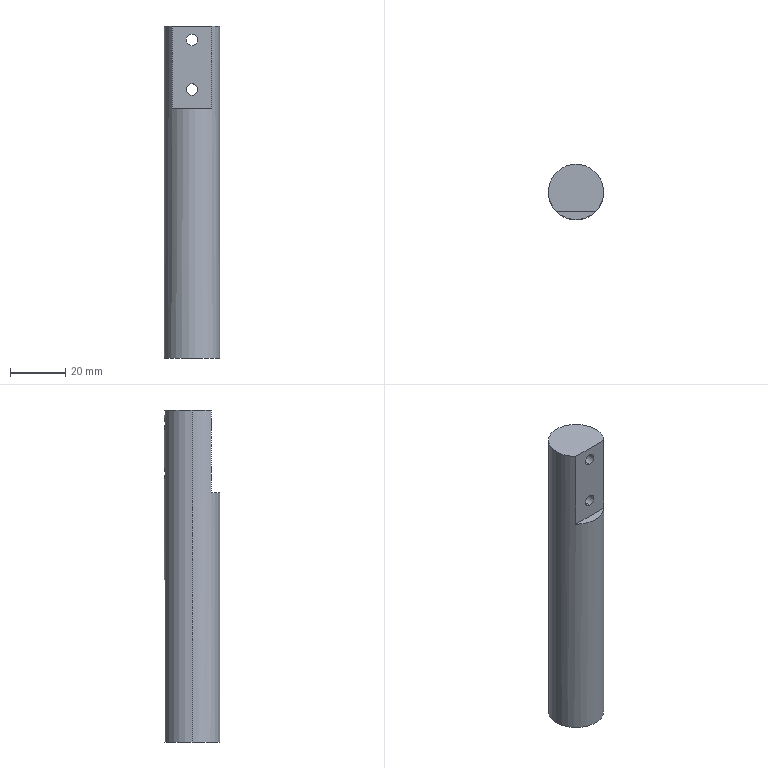Part | SolidWorks | features HoleWzd 2, Extrusion 1, ICE 1 | 1 solid | 14 faces | box 20 x 20 x 120 mm | volume 36039 mm3 | cylinder 8 | plane 4 | cone 2 | commonest cylinder face diameters 4.2 x4 5 x2 20 x2
STEP:
#1=CARTESIAN_POINT('',(0.,10.,57.1));
#2=VERTEX_POINT('',#1);
#3=CARTESIAN_POINT('',(0.,10.,52.9));
#4=VERTEX_POINT('',#3);
#5=CARTESIAN_POINT('',(0.,10.,57.1));
#6=CARTESIAN_POINT('',(-0.2745,10.,57.1));
#7=CARTESIAN_POINT('',(-0.5515,9.988,57.045));
#8=CARTESIAN_POINT('',(-0.9307,9.957,56.887));
#9=CARTESIAN_POINT('',(-1.053,9.945,56.822));
#10=CARTESIAN_POINT('',(-1.282,9.918,56.669));
#11=CARTESIAN_POINT('',(-1.387,9.904,56.582));
#12=CARTESIAN_POINT('',(-1.581,9.875,56.389));
#13=CARTESIAN_POINT('',(-1.669,9.86,56.281));
#14=CARTESIAN_POINT('',(-1.821,9.833,56.054));
#15=CARTESIAN_POINT('',(-1.886,9.821,55.934));
#16=CARTESIAN_POINT('',(-2.045,9.789,55.551));
#17=CARTESIAN_POINT('',(-2.1,9.777,55.278));
#18=CARTESIAN_POINT('',(-2.1,9.777,54.862));
#19=CARTESIAN_POINT('',(-2.087,9.78,54.726));
#20=CARTESIAN_POINT('',(-2.033,9.791,54.457));
#21=CARTESIAN_POINT('',(-1.992,9.8,54.323));
#22=CARTESIAN_POINT('',(-1.887,9.82,54.069));
#23=CARTESIAN_POINT('',(-1.823,9.833,53.948));
#24=CARTESIAN_POINT('',(-1.67,9.86,53.72));
#25=CARTESIAN_POINT('',(-1.582,9.875,53.613));
#26=CARTESIAN_POINT('',(-1.293,9.918,53.323));
#27=CARTESIAN_POINT('',(-1.06,9.947,53.166));
#28=CARTESIAN_POINT('',(-0.6807,9.978,53.009));
#29=CARTESIAN_POINT('',(-0.5474,9.986,52.968));
#30=CARTESIAN_POINT('',(-0.2764,9.997,52.914));
#31=CARTESIAN_POINT('',(-0.1391,10.,52.9));
#32=CARTESIAN_POINT('',(0.,10.,52.9));
#33=B_SPLINE_CURVE_WITH_KNOTS('',3,(#5,#6,#7,#8,#9,#10,#11,#12,#13,#14,#15,#16,#17,#18,#19,#20,#21,#22,#23,#24,#25,#26,#27,#28,#29,#30,#31,#32),.UNSPECIFIED.,.F.,.F.,(4,2,2,2,2,2,2,2,2,2,2,2,2,4),(0.006584,0.007407,0.007818,0.008229,0.008641,0.009052,0.009875,0.01029,0.0107,0.01111,0.01152,0.01234,0.01275,0.01317),.UNSPECIFIED.);
#34=EDGE_CURVE('',#2,#4,#33,.T.);
#35=ORIENTED_EDGE('',*,*,#34,.F.);
#36=CARTESIAN_POINT('',(0.,-7.,57.1));
#37=VERTEX_POINT('',#36);
#38=CARTESIAN_POINT('',(0.,-7.,57.1));
#39=DIRECTION('',(0.,-1.,0.));
#40=VECTOR('',#39,1000.);
#41=LINE('',#38,#40);
#42=EDGE_CURVE('',#2,#37,#41,.T.);
#43=ORIENTED_EDGE('',*,*,#42,.T.);
#44=CARTESIAN_POINT('',(0.,-7.,52.9));
#45=VERTEX_POINT('',#44);
#46=CARTESIAN_POINT('',(0.,-7.,55.));
#47=DIRECTION('',(0.,-1.,0.));
#48=DIRECTION('',(0.,0.,-1.));
#49=AXIS2_PLACEMENT_3D('',#46,#47,#48);
#50=CIRCLE('',#49,2.1);
#51=EDGE_CURVE('',#37,#45,#50,.T.);
#52=ORIENTED_EDGE('',*,*,#51,.T.);
#53=CARTESIAN_POINT('',(0.,-7.,52.9));
#54=DIRECTION('',(0.,-1.,0.));
#55=VECTOR('',#54,1000.);
#56=LINE('',#53,#55);
#57=EDGE_CURVE('',#4,#45,#56,.T.);
#58=ORIENTED_EDGE('',*,*,#57,.F.);
#59=EDGE_LOOP('',(#35,#43,#52,#58));
#60=FACE_OUTER_BOUND('',#59,.T.);
#61=CARTESIAN_POINT('',(0.,-7.,55.));
#62=DIRECTION('',(0.,-1.,0.));
#63=DIRECTION('',(0.,0.,-1.));
#64=AXIS2_PLACEMENT_3D('',#61,#62,#63);
#65=CYLINDRICAL_SURFACE('',#64,2.1);
#66=ADVANCED_FACE('',(#60),#65,.F.);
#67=CARTESIAN_POINT('',(0.,10.,39.1));
#68=VERTEX_POINT('',#67);
#69=CARTESIAN_POINT('',(0.,10.,34.9));
#70=VERTEX_POINT('',#69);
#71=CARTESIAN_POINT('',(0.,10.,39.1));
#72=CARTESIAN_POINT('',(-0.2745,10.,39.1));
#73=CARTESIAN_POINT('',(-0.5515,9.988,39.045));
#74=CARTESIAN_POINT('',(-0.9307,9.957,38.887));
#75=CARTESIAN_POINT('',(-1.053,9.945,38.822));
#76=CARTESIAN_POINT('',(-1.282,9.918,38.669));
#77=CARTESIAN_POINT('',(-1.387,9.904,38.582));
#78=CARTESIAN_POINT('',(-1.581,9.875,38.389));
#79=CARTESIAN_POINT('',(-1.669,9.86,38.281));
#80=CARTESIAN_POINT('',(-1.821,9.833,38.054));
#81=CARTESIAN_POINT('',(-1.886,9.821,37.934));
#82=CARTESIAN_POINT('',(-2.045,9.789,37.551));
#83=CARTESIAN_POINT('',(-2.1,9.777,37.278));
#84=CARTESIAN_POINT('',(-2.1,9.777,36.862));
#85=CARTESIAN_POINT('',(-2.087,9.78,36.726));
#86=CARTESIAN_POINT('',(-2.033,9.791,36.457));
#87=CARTESIAN_POINT('',(-1.992,9.8,36.323));
#88=CARTESIAN_POINT('',(-1.887,9.82,36.069));
#89=CARTESIAN_POINT('',(-1.823,9.833,35.948));
#90=CARTESIAN_POINT('',(-1.67,9.86,35.72));
#91=CARTESIAN_POINT('',(-1.582,9.875,35.613));
#92=CARTESIAN_POINT('',(-1.293,9.918,35.323));
#93=CARTESIAN_POINT('',(-1.06,9.947,35.166));
#94=CARTESIAN_POINT('',(-0.6807,9.978,35.009));
#95=CARTESIAN_POINT('',(-0.5474,9.986,34.968));
#96=CARTESIAN_POINT('',(-0.2764,9.997,34.914));
#97=CARTESIAN_POINT('',(-0.1391,10.,34.9));
#98=CARTESIAN_POINT('',(0.,10.,34.9));
#99=B_SPLINE_CURVE_WITH_KNOTS('',3,(#71,#72,#73,#74,#75,#76,#77,#78,#79,#80,#81,#82,#83,#84,#85,#86,#87,#88,#89,#90,#91,#92,#93,#94,#95,#96,#97,#98),.UNSPECIFIED.,.F.,.F.,(4,2,2,2,2,2,2,2,2,2,2,2,2,4),(0.006584,0.007407,0.007818,0.008229,0.008641,0.009052,0.009875,0.01029,0.0107,0.01111,0.01152,0.01234,0.01275,0.01317),.UNSPECIFIED.);
#100=EDGE_CURVE('',#68,#70,#99,.T.);
#101=ORIENTED_EDGE('',*,*,#100,.F.);
#102=CARTESIAN_POINT('',(0.,-7.,39.1));
#103=VERTEX_POINT('',#102);
#104=CARTESIAN_POINT('',(0.,-7.,39.1));
#105=DIRECTION('',(0.,-1.,0.));
#106=VECTOR('',#105,1000.);
#107=LINE('',#104,#106);
#108=EDGE_CURVE('',#68,#103,#107,.T.);
#109=ORIENTED_EDGE('',*,*,#108,.T.);
#110=CARTESIAN_POINT('',(0.,-7.,34.9));
#111=VERTEX_POINT('',#110);
#112=CARTESIAN_POINT('',(0.,-7.,37.));
#113=DIRECTION('',(0.,-1.,0.));
#114=DIRECTION('',(0.,0.,-1.));
#115=AXIS2_PLACEMENT_3D('',#112,#113,#114);
#116=CIRCLE('',#115,2.1);
#117=EDGE_CURVE('',#103,#111,#116,.T.);
#118=ORIENTED_EDGE('',*,*,#117,.T.);
#119=CARTESIAN_POINT('',(0.,-7.,34.9));
#120=DIRECTION('',(0.,-1.,0.));
#121=VECTOR('',#120,1000.);
#122=LINE('',#119,#121);
#123=EDGE_CURVE('',#70,#111,#122,.T.);
#124=ORIENTED_EDGE('',*,*,#123,.F.);
#125=EDGE_LOOP('',(#101,#109,#118,#124));
#126=FACE_OUTER_BOUND('',#125,.T.);
#127=CARTESIAN_POINT('',(0.,-7.,37.));
#128=DIRECTION('',(0.,-1.,0.));
#129=DIRECTION('',(0.,0.,-1.));
#130=AXIS2_PLACEMENT_3D('',#127,#128,#129);
#131=CYLINDRICAL_SURFACE('',#130,2.1);
#132=ADVANCED_FACE('',(#126),#131,.F.);
#133=CARTESIAN_POINT('',(2.5,0.,-45.));
#134=VERTEX_POINT('',#133);
#135=CARTESIAN_POINT('',(-2.5,0.,-45.));
#136=VERTEX_POINT('',#135);
#137=CARTESIAN_POINT('',(0.,0.,-45.));
#138=DIRECTION('',(0.,0.,-1.));
#139=DIRECTION('',(-1.,0.,0.));
#140=AXIS2_PLACEMENT_3D('',#137,#138,#139);
#141=CIRCLE('',#140,2.5);
#142=EDGE_CURVE('',#134,#136,#141,.T.);
#143=ORIENTED_EDGE('',*,*,#142,.F.);
#144=CARTESIAN_POINT('',(2.5,0.,-60.));
#145=VERTEX_POINT('',#144);
#146=CARTESIAN_POINT('',(2.5,0.,-60.));
#147=DIRECTION('',(0.,0.,-1.));
#148=VECTOR('',#147,1000.);
#149=LINE('',#146,#148);
#150=EDGE_CURVE('',#134,#145,#149,.T.);
#151=ORIENTED_EDGE('',*,*,#150,.T.);
#152=CARTESIAN_POINT('',(-2.5,0.,-60.));
#153=VERTEX_POINT('',#152);
#154=CARTESIAN_POINT('',(0.,0.,-60.));
#155=DIRECTION('',(0.,0.,-1.));
#156=DIRECTION('',(-1.,0.,0.));
#157=AXIS2_PLACEMENT_3D('',#154,#155,#156);
#158=CIRCLE('',#157,2.5);
#159=EDGE_CURVE('',#145,#153,#158,.T.);
#160=ORIENTED_EDGE('',*,*,#159,.T.);
#161=CARTESIAN_POINT('',(-2.5,0.,-60.));
#162=DIRECTION('',(0.,0.,-1.));
#163=VECTOR('',#162,1000.);
#164=LINE('',#161,#163);
#165=EDGE_CURVE('',#136,#153,#164,.T.);
#166=ORIENTED_EDGE('',*,*,#165,.F.);
#167=EDGE_LOOP('',(#143,#151,#160,#166));
#168=FACE_OUTER_BOUND('',#167,.T.);
#169=CARTESIAN_POINT('',(0.,0.,-60.));
#170=DIRECTION('',(0.,0.,-1.));
#171=DIRECTION('',(-1.,0.,0.));
#172=AXIS2_PLACEMENT_3D('',#169,#170,#171);
#173=CYLINDRICAL_SURFACE('',#172,2.5);
#174=ADVANCED_FACE('',(#168),#173,.F.);
#175=CARTESIAN_POINT('',(0.,0.,-43.498));
#176=VERTEX_POINT('',#175);
#177=CARTESIAN_POINT('',(-2.5,0.,-45.));
#178=DIRECTION('',(-0.8572,0.,-0.515));
#179=VECTOR('',#178,1000.);
#180=LINE('',#177,#179);
#181=EDGE_CURVE('',#176,#136,#180,.T.);
#182=ORIENTED_EDGE('',*,*,#181,.F.);
#183=CARTESIAN_POINT('',(2.5,0.,-45.));
#184=DIRECTION('',(0.8572,0.,-0.515));
#185=VECTOR('',#184,1000.);
#186=LINE('',#183,#185);
#187=EDGE_CURVE('',#176,#134,#186,.T.);
#188=ORIENTED_EDGE('',*,*,#187,.T.);
#189=ORIENTED_EDGE('',*,*,#142,.T.);
#190=EDGE_LOOP('',(#182,#188,#189));
#191=FACE_OUTER_BOUND('',#190,.T.);
#192=CARTESIAN_POINT('',(0.,0.,-45.));
#193=DIRECTION('',(0.,0.,-1.));
#194=DIRECTION('',(-1.,0.,0.));
#195=AXIS2_PLACEMENT_3D('',#192,#193,#194);
#196=CONICAL_SURFACE('',#195,2.5,1.03);
#197=ADVANCED_FACE('',(#191),#196,.F.);
#198=CARTESIAN_POINT('',(0.,10.,52.9));
#199=CARTESIAN_POINT('',(0.1392,10.,52.9));
#200=CARTESIAN_POINT('',(0.2759,9.997,52.914));
#201=CARTESIAN_POINT('',(0.5449,9.986,52.967));
#202=CARTESIAN_POINT('',(0.6785,9.978,53.008));
#203=CARTESIAN_POINT('',(0.9326,9.957,53.113));
#204=CARTESIAN_POINT('',(1.053,9.945,53.178));
#205=CARTESIAN_POINT('',(1.281,9.918,53.33));
#206=CARTESIAN_POINT('',(1.389,9.904,53.419));
#207=CARTESIAN_POINT('',(1.678,9.86,53.709));
#208=CARTESIAN_POINT('',(1.835,9.831,53.942));
#209=CARTESIAN_POINT('',(1.992,9.8,54.321));
#210=CARTESIAN_POINT('',(2.032,9.791,54.454));
#211=CARTESIAN_POINT('',(2.087,9.78,54.725));
#212=CARTESIAN_POINT('',(2.1,9.777,54.862));
#213=CARTESIAN_POINT('',(2.1,9.777,55.137));
#214=CARTESIAN_POINT('',(2.086,9.78,55.276));
#215=CARTESIAN_POINT('',(2.032,9.791,55.546));
#216=CARTESIAN_POINT('',(1.993,9.8,55.677));
#217=CARTESIAN_POINT('',(1.834,9.831,56.059));
#218=CARTESIAN_POINT('',(1.68,9.86,56.29));
#219=CARTESIAN_POINT('',(1.387,9.904,56.583));
#220=CARTESIAN_POINT('',(1.282,9.918,56.669));
#221=CARTESIAN_POINT('',(1.054,9.945,56.821));
#222=CARTESIAN_POINT('',(0.9314,9.957,56.887));
#223=CARTESIAN_POINT('',(0.6776,9.978,56.992));
#224=CARTESIAN_POINT('',(0.5467,9.986,57.032));
#225=CARTESIAN_POINT('',(0.2767,9.997,57.086));
#226=CARTESIAN_POINT('',(0.1373,10.,57.1));
#227=CARTESIAN_POINT('',(0.,10.,57.1));
#228=B_SPLINE_CURVE_WITH_KNOTS('',3,(#198,#199,#200,#201,#202,#203,#204,#205,#206,#207,#208,#209,#210,#211,#212,#213,#214,#215,#216,#217,#218,#219,#220,#221,#222,#223,#224,#225,#226,#227),.UNSPECIFIED.,.F.,.F.,(4,2,2,2,2,2,2,2,2,2,2,2,2,2,4),(0.,0.0004115,0.000823,0.001234,0.001646,0.002469,0.00288,0.003292,0.003703,0.004115,0.004938,0.005349,0.005761,0.006172,0.006584),.UNSPECIFIED.);
#229=EDGE_CURVE('',#4,#2,#228,.T.);
#230=ORIENTED_EDGE('',*,*,#229,.T.);
#231=ORIENTED_EDGE('',*,*,#34,.T.);
#232=EDGE_LOOP('',(#230,#231));
#233=FACE_BOUND('',#232,.T.);
#234=CARTESIAN_POINT('',(0.,10.,34.9));
#235=CARTESIAN_POINT('',(0.1392,10.,34.9));
#236=CARTESIAN_POINT('',(0.2759,9.997,34.914));
#237=CARTESIAN_POINT('',(0.5449,9.986,34.967));
#238=CARTESIAN_POINT('',(0.6785,9.978,35.008));
#239=CARTESIAN_POINT('',(0.9326,9.957,35.113));
#240=CARTESIAN_POINT('',(1.053,9.945,35.178));
#241=CARTESIAN_POINT('',(1.281,9.918,35.33));
#242=CARTESIAN_POINT('',(1.389,9.904,35.419));
#243=CARTESIAN_POINT('',(1.678,9.86,35.709));
#244=CARTESIAN_POINT('',(1.835,9.831,35.942));
#245=CARTESIAN_POINT('',(1.992,9.8,36.321));
#246=CARTESIAN_POINT('',(2.032,9.791,36.454));
#247=CARTESIAN_POINT('',(2.087,9.78,36.725));
#248=CARTESIAN_POINT('',(2.1,9.777,36.862));
#249=CARTESIAN_POINT('',(2.1,9.777,37.137));
#250=CARTESIAN_POINT('',(2.086,9.78,37.276));
#251=CARTESIAN_POINT('',(2.032,9.791,37.546));
#252=CARTESIAN_POINT('',(1.993,9.8,37.677));
#253=CARTESIAN_POINT('',(1.834,9.831,38.059));
#254=CARTESIAN_POINT('',(1.68,9.86,38.29));
#255=CARTESIAN_POINT('',(1.387,9.904,38.583));
#256=CARTESIAN_POINT('',(1.282,9.918,38.669));
#257=CARTESIAN_POINT('',(1.054,9.945,38.821));
#258=CARTESIAN_POINT('',(0.9314,9.957,38.887));
#259=CARTESIAN_POINT('',(0.6776,9.978,38.992));
#260=CARTESIAN_POINT('',(0.5467,9.986,39.032));
#261=CARTESIAN_POINT('',(0.2767,9.997,39.086));
#262=CARTESIAN_POINT('',(0.1373,10.,39.1));
#263=CARTESIAN_POINT('',(0.,10.,39.1));
#264=B_SPLINE_CURVE_WITH_KNOTS('',3,(#234,#235,#236,#237,#238,#239,#240,#241,#242,#243,#244,#245,#246,#247,#248,#249,#250,#251,#252,#253,#254,#255,#256,#257,#258,#259,#260,#261,#262,#263),.UNSPECIFIED.,.F.,.F.,(4,2,2,2,2,2,2,2,2,2,2,2,2,2,4),(0.,0.0004115,0.000823,0.001234,0.001646,0.002469,0.00288,0.003292,0.003703,0.004115,0.004938,0.005349,0.005761,0.006172,0.006584),.UNSPECIFIED.);
#265=EDGE_CURVE('',#70,#68,#264,.T.);
#266=ORIENTED_EDGE('',*,*,#265,.T.);
#267=ORIENTED_EDGE('',*,*,#100,.T.);
#268=EDGE_LOOP('',(#266,#267));
#269=FACE_BOUND('',#268,.T.);
#270=CARTESIAN_POINT('',(10.,0.,60.));
#271=VERTEX_POINT('',#270);
#272=CARTESIAN_POINT('',(-10.,0.,60.));
#273=VERTEX_POINT('',#272);
#274=CARTESIAN_POINT('',(0.,0.,60.));
#275=DIRECTION('',(0.,0.,1.));
#276=DIRECTION('',(1.,0.,0.));
#277=AXIS2_PLACEMENT_3D('',#274,#275,#276);
#278=CIRCLE('',#277,10.);
#279=EDGE_CURVE('',#271,#273,#278,.T.);
#280=ORIENTED_EDGE('',*,*,#279,.F.);
#281=CARTESIAN_POINT('',(10.,0.,-60.));
#282=VERTEX_POINT('',#281);
#283=CARTESIAN_POINT('',(10.,0.,60.));
#284=DIRECTION('',(0.,0.,-1.));
#285=VECTOR('',#284,1000.);
#286=LINE('',#283,#285);
#287=EDGE_CURVE('',#271,#282,#286,.T.);
#288=ORIENTED_EDGE('',*,*,#287,.T.);
#289=CARTESIAN_POINT('',(-10.,0.,-60.));
#290=VERTEX_POINT('',#289);
#291=CARTESIAN_POINT('',(0.,0.,-60.));
#292=DIRECTION('',(0.,0.,1.));
#293=DIRECTION('',(1.,0.,0.));
#294=AXIS2_PLACEMENT_3D('',#291,#292,#293);
#295=CIRCLE('',#294,10.);
#296=EDGE_CURVE('',#282,#290,#295,.T.);
#297=ORIENTED_EDGE('',*,*,#296,.T.);
#298=CARTESIAN_POINT('',(-10.,0.,60.));
#299=DIRECTION('',(0.,0.,-1.));
#300=VECTOR('',#299,1000.);
#301=LINE('',#298,#300);
#302=EDGE_CURVE('',#273,#290,#301,.T.);
#303=ORIENTED_EDGE('',*,*,#302,.F.);
#304=EDGE_LOOP('',(#280,#288,#297,#303));
#305=FACE_OUTER_BOUND('',#304,.T.);
#306=CARTESIAN_POINT('',(0.,0.,60.));
#307=DIRECTION('',(0.,0.,-1.));
#308=DIRECTION('',(-1.,0.,0.));
#309=AXIS2_PLACEMENT_3D('',#306,#307,#308);
#310=CYLINDRICAL_SURFACE('',#309,10.);
#311=ADVANCED_FACE('',(#233,#269,#305),#310,.T.);
#312=ORIENTED_EDGE('',*,*,#287,.F.);
#313=CARTESIAN_POINT('',(7.141,-7.,60.));
#314=VERTEX_POINT('',#313);
#315=CARTESIAN_POINT('',(0.,0.,60.));
#316=DIRECTION('',(0.,0.,1.));
#317=DIRECTION('',(1.,0.,0.));
#318=AXIS2_PLACEMENT_3D('',#315,#316,#317);
#319=CIRCLE('',#318,10.);
#320=EDGE_CURVE('',#314,#271,#319,.T.);
#321=ORIENTED_EDGE('',*,*,#320,.F.);
#322=CARTESIAN_POINT('',(7.141,-7.,30.));
#323=VERTEX_POINT('',#322);
#324=CARTESIAN_POINT('',(7.141,-7.,30.));
#325=DIRECTION('',(0.,0.,1.));
#326=VECTOR('',#325,1000.);
#327=LINE('',#324,#326);
#328=EDGE_CURVE('',#323,#314,#327,.T.);
#329=ORIENTED_EDGE('',*,*,#328,.F.);
#330=CARTESIAN_POINT('',(-7.141,-7.,30.));
#331=VERTEX_POINT('',#330);
#332=CARTESIAN_POINT('',(0.,0.,30.));
#333=DIRECTION('',(0.,0.,1.));
#334=DIRECTION('',(1.,0.,0.));
#335=AXIS2_PLACEMENT_3D('',#332,#333,#334);
#336=CIRCLE('',#335,10.);
#337=EDGE_CURVE('',#331,#323,#336,.T.);
#338=ORIENTED_EDGE('',*,*,#337,.F.);
#339=CARTESIAN_POINT('',(-7.141,-7.,60.));
#340=VERTEX_POINT('',#339);
#341=CARTESIAN_POINT('',(-7.141,-7.,30.));
#342=DIRECTION('',(0.,0.,1.));
#343=VECTOR('',#342,1000.);
#344=LINE('',#341,#343);
#345=EDGE_CURVE('',#331,#340,#344,.T.);
#346=ORIENTED_EDGE('',*,*,#345,.T.);
#347=CARTESIAN_POINT('',(0.,0.,60.));
#348=DIRECTION('',(0.,0.,1.));
#349=DIRECTION('',(1.,0.,0.));
#350=AXIS2_PLACEMENT_3D('',#347,#348,#349);
#351=CIRCLE('',#350,10.);
#352=EDGE_CURVE('',#273,#340,#351,.T.);
#353=ORIENTED_EDGE('',*,*,#352,.F.);
#354=ORIENTED_EDGE('',*,*,#302,.T.);
#355=CARTESIAN_POINT('',(0.,0.,-60.));
#356=DIRECTION('',(0.,0.,1.));
#357=DIRECTION('',(1.,0.,0.));
#358=AXIS2_PLACEMENT_3D('',#355,#356,#357);
#359=CIRCLE('',#358,10.);
#360=EDGE_CURVE('',#290,#282,#359,.T.);
#361=ORIENTED_EDGE('',*,*,#360,.T.);
#362=EDGE_LOOP('',(#312,#321,#329,#338,#346,#353,#354,#361));
#363=FACE_OUTER_BOUND('',#362,.T.);
#364=CARTESIAN_POINT('',(0.,0.,60.));
#365=DIRECTION('',(0.,0.,-1.));
#366=DIRECTION('',(-1.,0.,0.));
#367=AXIS2_PLACEMENT_3D('',#364,#365,#366);
#368=CYLINDRICAL_SURFACE('',#367,10.);
#369=ADVANCED_FACE('',(#363),#368,.T.);
#370=CARTESIAN_POINT('',(7.141,-7.,60.));
#371=DIRECTION('',(-1.,0.,0.));
#372=VECTOR('',#371,1000.);
#373=LINE('',#370,#372);
#374=EDGE_CURVE('',#314,#340,#373,.T.);
#375=ORIENTED_EDGE('',*,*,#374,.F.);
#376=ORIENTED_EDGE('',*,*,#320,.T.);
#377=ORIENTED_EDGE('',*,*,#279,.T.);
#378=ORIENTED_EDGE('',*,*,#352,.T.);
#379=EDGE_LOOP('',(#375,#376,#377,#378));
#380=FACE_OUTER_BOUND('',#379,.T.);
#381=CARTESIAN_POINT('',(0.,0.,60.));
#382=DIRECTION('',(0.,0.,1.));
#383=DIRECTION('',(1.,0.,0.));
#384=AXIS2_PLACEMENT_3D('',#381,#382,#383);
#385=PLANE('',#384);
#386=ADVANCED_FACE('',(#380),#385,.T.);
#387=CARTESIAN_POINT('',(0.,0.,-60.));
#388=DIRECTION('',(0.,0.,-1.));
#389=DIRECTION('',(-1.,0.,0.));
#390=AXIS2_PLACEMENT_3D('',#387,#388,#389);
#391=CIRCLE('',#390,2.5);
#392=EDGE_CURVE('',#153,#145,#391,.T.);
#393=ORIENTED_EDGE('',*,*,#392,.F.);
#394=ORIENTED_EDGE('',*,*,#159,.F.);
#395=EDGE_LOOP('',(#393,#394));
#396=FACE_BOUND('',#395,.T.);
#397=ORIENTED_EDGE('',*,*,#360,.F.);
#398=ORIENTED_EDGE('',*,*,#296,.F.);
#399=EDGE_LOOP('',(#397,#398));
#400=FACE_OUTER_BOUND('',#399,.T.);
#401=CARTESIAN_POINT('',(0.,0.,-60.));
#402=DIRECTION('',(0.,0.,1.));
#403=DIRECTION('',(1.,0.,0.));
#404=AXIS2_PLACEMENT_3D('',#401,#402,#403);
#405=PLANE('',#404);
#406=ADVANCED_FACE('',(#396,#400),#405,.F.);
#407=ORIENTED_EDGE('',*,*,#187,.F.);
#408=ORIENTED_EDGE('',*,*,#181,.T.);
#409=CARTESIAN_POINT('',(0.,0.,-45.));
#410=DIRECTION('',(0.,0.,-1.));
#411=DIRECTION('',(-1.,0.,0.));
#412=AXIS2_PLACEMENT_3D('',#409,#410,#411);
#413=CIRCLE('',#412,2.5);
#414=EDGE_CURVE('',#136,#134,#413,.T.);
#415=ORIENTED_EDGE('',*,*,#414,.T.);
#416=EDGE_LOOP('',(#407,#408,#415));
#417=FACE_OUTER_BOUND('',#416,.T.);
#418=CARTESIAN_POINT('',(0.,0.,-45.));
#419=DIRECTION('',(0.,0.,-1.));
#420=DIRECTION('',(-1.,0.,0.));
#421=AXIS2_PLACEMENT_3D('',#418,#419,#420);
#422=CONICAL_SURFACE('',#421,2.5,1.03);
#423=ADVANCED_FACE('',(#417),#422,.F.);
#424=ORIENTED_EDGE('',*,*,#150,.F.);
#425=ORIENTED_EDGE('',*,*,#414,.F.);
#426=ORIENTED_EDGE('',*,*,#165,.T.);
#427=ORIENTED_EDGE('',*,*,#392,.T.);
#428=EDGE_LOOP('',(#424,#425,#426,#427));
#429=FACE_OUTER_BOUND('',#428,.T.);
#430=CARTESIAN_POINT('',(0.,0.,-60.));
#431=DIRECTION('',(0.,0.,-1.));
#432=DIRECTION('',(-1.,0.,0.));
#433=AXIS2_PLACEMENT_3D('',#430,#431,#432);
#434=CYLINDRICAL_SURFACE('',#433,2.5);
#435=ADVANCED_FACE('',(#429),#434,.F.);
#436=ORIENTED_EDGE('',*,*,#337,.T.);
#437=CARTESIAN_POINT('',(7.141,-7.,30.));
#438=DIRECTION('',(-1.,0.,0.));
#439=VECTOR('',#438,1000.);
#440=LINE('',#437,#439);
#441=EDGE_CURVE('',#323,#331,#440,.T.);
#442=ORIENTED_EDGE('',*,*,#441,.T.);
#443=EDGE_LOOP('',(#436,#442));
#444=FACE_OUTER_BOUND('',#443,.T.);
#445=CARTESIAN_POINT('',(0.,0.,30.));
#446=DIRECTION('',(0.,0.,1.));
#447=DIRECTION('',(1.,0.,0.));
#448=AXIS2_PLACEMENT_3D('',#445,#446,#447);
#449=PLANE('',#448);
#450=ADVANCED_FACE('',(#444),#449,.T.);
#451=CARTESIAN_POINT('',(0.,-7.,55.));
#452=DIRECTION('',(0.,-1.,0.));
#453=DIRECTION('',(0.,0.,-1.));
#454=AXIS2_PLACEMENT_3D('',#451,#452,#453);
#455=CIRCLE('',#454,2.1);
#456=EDGE_CURVE('',#45,#37,#455,.T.);
#457=ORIENTED_EDGE('',*,*,#456,.F.);
#458=ORIENTED_EDGE('',*,*,#51,.F.);
#459=EDGE_LOOP('',(#457,#458));
#460=FACE_BOUND('',#459,.T.);
#461=CARTESIAN_POINT('',(0.,-7.,37.));
#462=DIRECTION('',(0.,-1.,0.));
#463=DIRECTION('',(0.,0.,-1.));
#464=AXIS2_PLACEMENT_3D('',#461,#462,#463);
#465=CIRCLE('',#464,2.1);
#466=EDGE_CURVE('',#111,#103,#465,.T.);
#467=ORIENTED_EDGE('',*,*,#466,.F.);
#468=ORIENTED_EDGE('',*,*,#117,.F.);
#469=EDGE_LOOP('',(#467,#468));
#470=FACE_BOUND('',#469,.T.);
#471=ORIENTED_EDGE('',*,*,#374,.T.);
#472=ORIENTED_EDGE('',*,*,#345,.F.);
#473=ORIENTED_EDGE('',*,*,#441,.F.);
#474=ORIENTED_EDGE('',*,*,#328,.T.);
#475=EDGE_LOOP('',(#471,#472,#473,#474));
#476=FACE_OUTER_BOUND('',#475,.T.);
#477=CARTESIAN_POINT('',(7.141,-7.,30.));
#478=DIRECTION('',(0.,1.,0.));
#479=DIRECTION('',(0.,0.,1.));
#480=AXIS2_PLACEMENT_3D('',#477,#478,#479);
#481=PLANE('',#480);
#482=ADVANCED_FACE('',(#460,#470,#476),#481,.F.);
#483=ORIENTED_EDGE('',*,*,#108,.F.);
#484=ORIENTED_EDGE('',*,*,#265,.F.);
#485=ORIENTED_EDGE('',*,*,#123,.T.);
#486=ORIENTED_EDGE('',*,*,#466,.T.);
#487=EDGE_LOOP('',(#483,#484,#485,#486));
#488=FACE_OUTER_BOUND('',#487,.T.);
#489=CARTESIAN_POINT('',(0.,-7.,37.));
#490=DIRECTION('',(0.,-1.,0.));
#491=DIRECTION('',(0.,0.,-1.));
#492=AXIS2_PLACEMENT_3D('',#489,#490,#491);
#493=CYLINDRICAL_SURFACE('',#492,2.1);
#494=ADVANCED_FACE('',(#488),#493,.F.);
#495=ORIENTED_EDGE('',*,*,#42,.F.);
#496=ORIENTED_EDGE('',*,*,#229,.F.);
#497=ORIENTED_EDGE('',*,*,#57,.T.);
#498=ORIENTED_EDGE('',*,*,#456,.T.);
#499=EDGE_LOOP('',(#495,#496,#497,#498));
#500=FACE_OUTER_BOUND('',#499,.T.);
#501=CARTESIAN_POINT('',(0.,-7.,55.));
#502=DIRECTION('',(0.,-1.,0.));
#503=DIRECTION('',(0.,0.,-1.));
#504=AXIS2_PLACEMENT_3D('',#501,#502,#503);
#505=CYLINDRICAL_SURFACE('',#504,2.1);
#506=ADVANCED_FACE('',(#500),#505,.F.);
#507=CLOSED_SHELL('',(#66,#132,#174,#197,#311,#369,#386,#406,#423,#435,#450,#482,#494,#506));
#508=MANIFOLD_SOLID_BREP('',#507);
#509=CARTESIAN_POINT('',(0.,0.,0.));
#510=DIRECTION('',(0.,0.,1.));
#511=DIRECTION('',(1.,0.,0.));
#512=AXIS2_PLACEMENT_3D('',#509,#510,#511);
#513=(LENGTH_UNIT()NAMED_UNIT(*)SI_UNIT(.MILLI.,.METRE.));
#514=UNCERTAINTY_MEASURE_WITH_UNIT(LENGTH_MEASURE(0.00001),#513,'','');
#515=(NAMED_UNIT(*)PLANE_ANGLE_UNIT()SI_UNIT($,.RADIAN.));
#516=(NAMED_UNIT(*)SI_UNIT($,.STERADIAN.)SOLID_ANGLE_UNIT());
#517=(GEOMETRIC_REPRESENTATION_CONTEXT(3)GLOBAL_UNCERTAINTY_ASSIGNED_CONTEXT((#514))GLOBAL_UNIT_ASSIGNED_CONTEXT((#513,#515,#516))REPRESENTATION_CONTEXT('',''));
#518=ADVANCED_BREP_SHAPE_REPRESENTATION('',(#508,#512),#517);